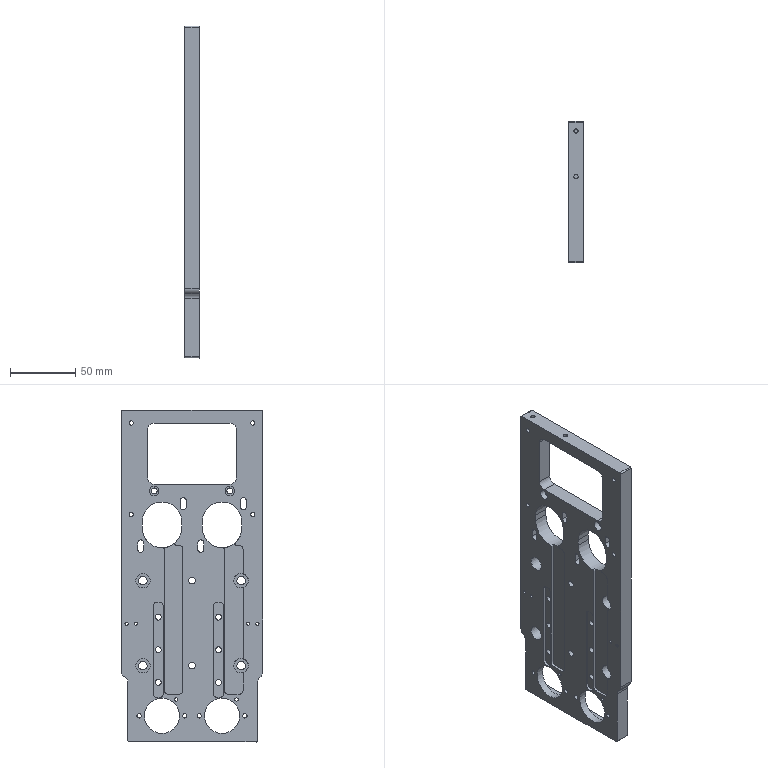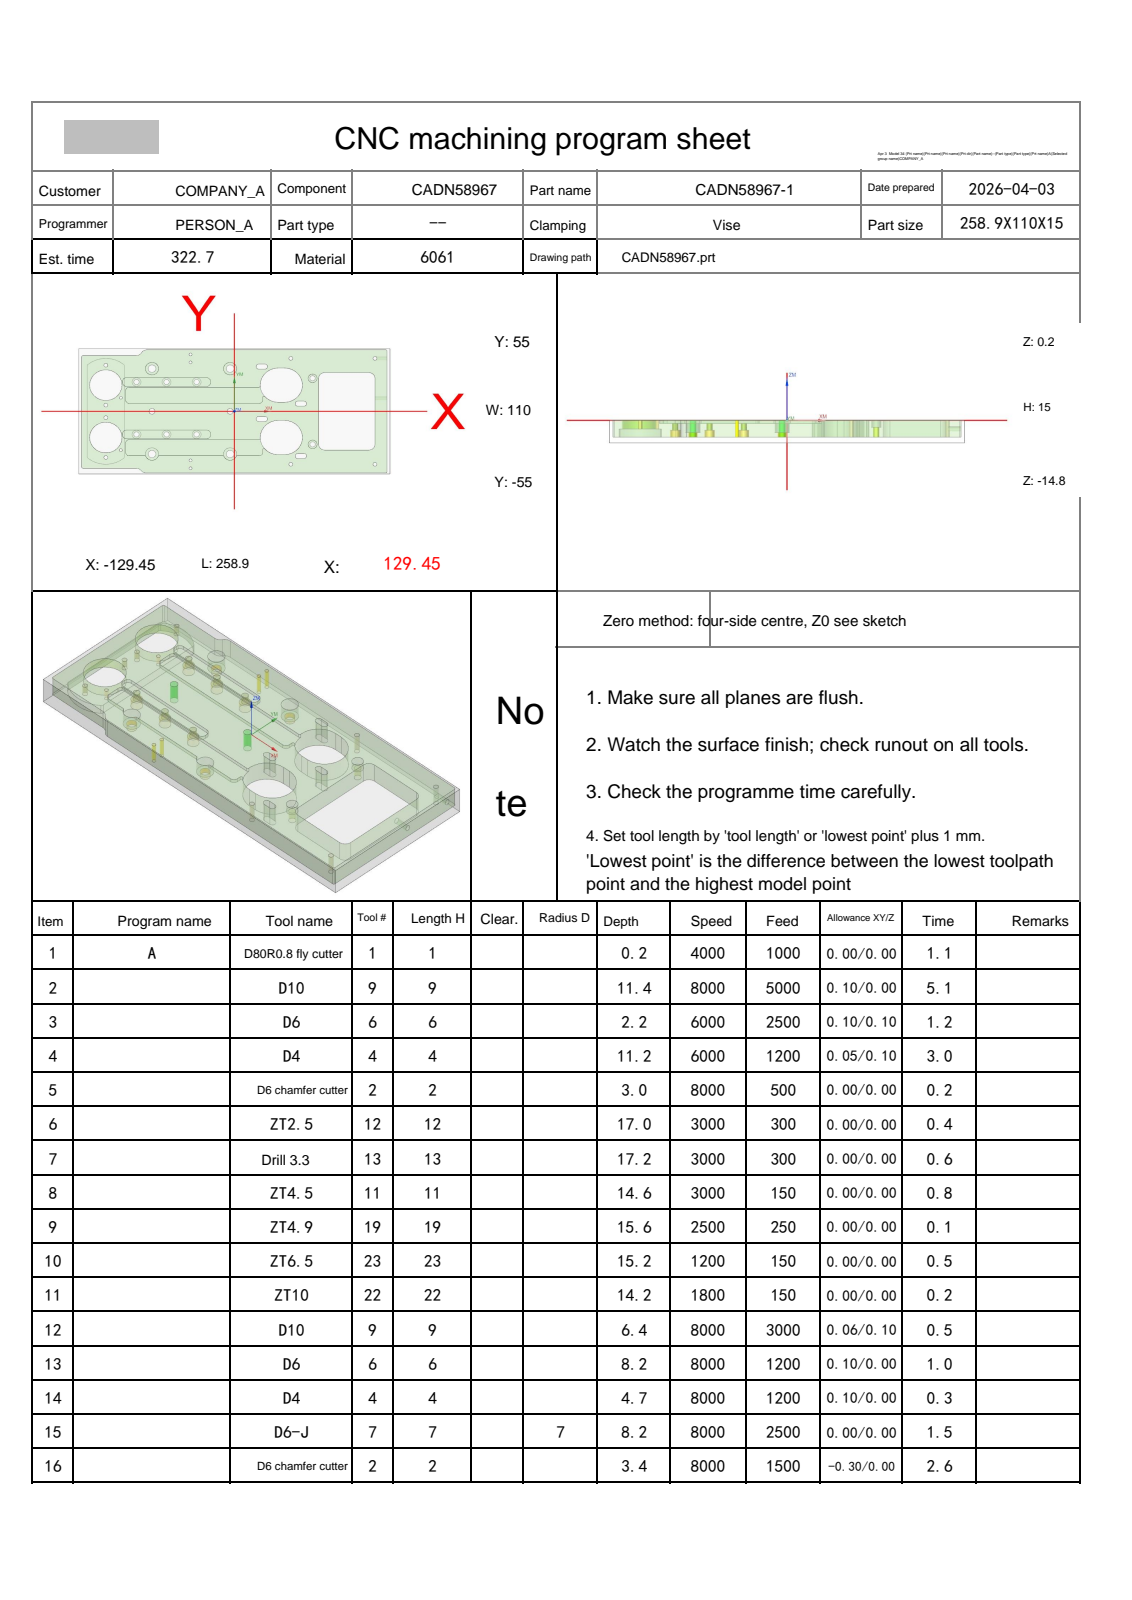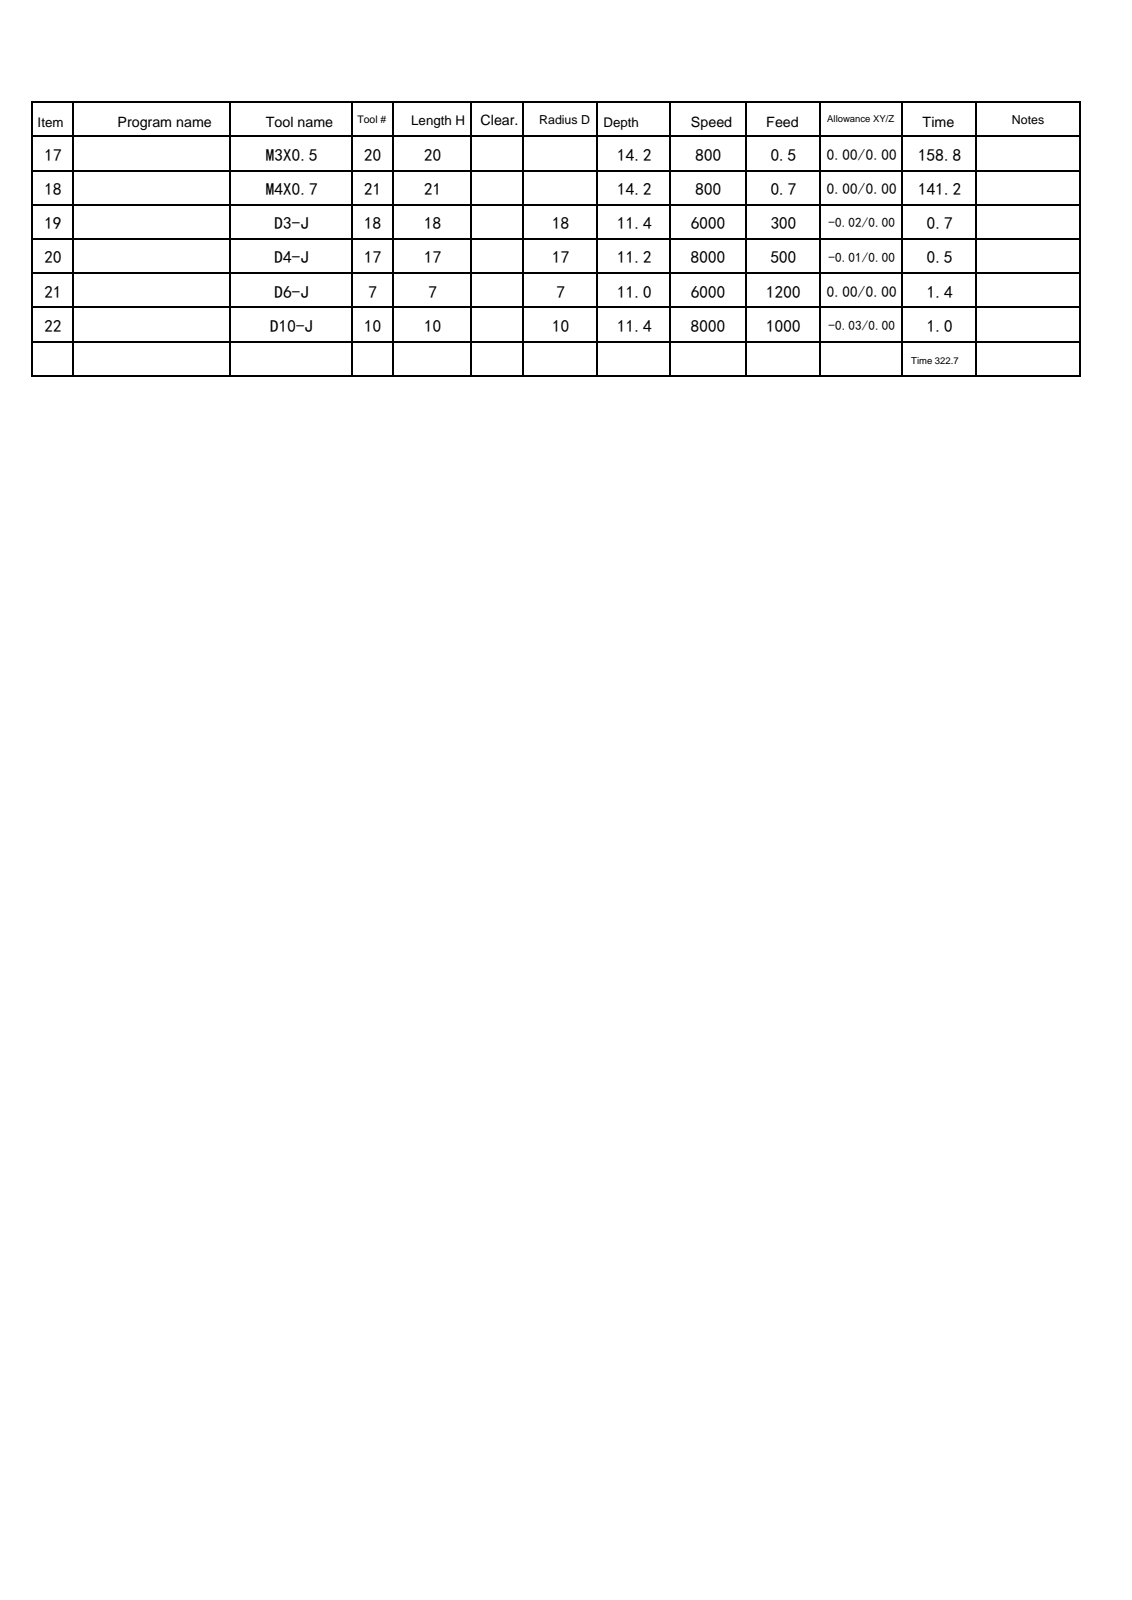NC program | NX | posted by the shop | part box 11 x 108 x 253.9 mm
Lines 1 to 910 of 8037:
%
O0001
(Machine time: 603.29 MIN)
(===Total Tool:17===)
(T1=D80R0.8 fly cutter D=80.  R=0.8  D-  H01 Z=0.    )
(T9=D10     D=10.  R=0.   D-  H09 Z=-11.2 )
(T6=D6      D=6.   R=0.   D-  H06 Z=-8.   )
(T4=D4      D=4.   R=0.   D-  H04 Z=-11.  )
(T2=D6 chamfer cutter   D=6.   R=0.   D-  H02 Z=-3.2  )
(T12=ZT2.5  D=2.5  DR_a=118 D-  H12 Z=-16.75)
(T13=drill 3.3  D=3.3  DR_a=118 D-  H13 Z=-17.  )
(T11=ZT4.5  D=4.5  DR_a=118 D-  H11 Z=-14.35)
(T19=ZT4.9  D=4.9  DR_a=120 D-  H19 Z=-15.41)
(T23=ZT6.5  D=6.5  DR_a=118 D-  H23 Z=-14.95)
(T22=ZT10   D=10.  DR_a=118 D-  H22 Z=-14.  )
(T7=D6-J    D=6.   R=0.   D7  H07 Z=-10.85)
(T20=M3X0.5 D=2.5  DR_a=180 D-  H20 Z=-14.  )
(T21=M4X0.7 D=3.3  DR_a=180 D-  H21 Z=-14.  )
(T18=D3-J   D=3.   R=0.   D18 H18 Z=-11.2 )
(T17=D4-J   D=4.   R=0.   D17 H17 Z=-11.  )
(T10=D10-J  D=10.  R=0.   D10 H10 Z=-11.2 )
G80 G90 G17 G49 G40
G91 G28 Z0
M01
N1 T01 M06
(D80R0.8 fly cutter  D=80. R=0.8 H=01 ce=0.00 di=0.00)
G00 G90 G54 X-171.95 Y47. M03 S4000
G43 H01 Z20.
M08
Z2.
G01 Z0.0 F1000.
X-166.95
X166.95
Y0.0
X-166.95
Y-47.
X166.95
X171.95
Z2.
G00 Z20.
G91 G28 Z0.0
M05
M09
G91 G28 Z0.0
M01
N2 T09 M06
(D10  D=10. R=0. H=09 ce=0.10 di=0.00)
G00 G90 G54 X26.2 Y-59.1 M03 S8000
G43 H09 Z20.
M08
Z.5
G01 X-73.55 Z.396 F5000.
G02 X-81.6 Y-55.1 Z.386 I0.0 J10.1
G01 X-125.95 Z.34
G02 X-132.05 Y-49. Z.33 I0.0 J6.1
G01 Y48. Z.229
G02 X-125.95 Y54.1 Z.219 I6.1 J0.0
G01 X-81.608 Z.173
G02 X-72.89 Y59.1 Z.162 I8.718 J-5.1
G01 X125.95 Z-.046
G02 X132.05 Y53. Z-.056 I0.0 J-6.1
G01 Y-53. Z-.166
G02 X125.95 Y-59.1 Z-.176 I-6.1 J0.0
G01 X-73.55 Z-.384
G02 X-81.6 Y-55.1 Z-.394 I0.0 J10.1
G01 X-125.95 Z-.44
G02 X-132.05 Y-49. Z-.45 I0.0 J6.1
G01 Y48. Z-.551
G02 X-125.95 Y54.1 Z-.561 I6.1 J0.0
G01 X-81.608 Z-.607
G02 X-72.89 Y59.1 Z-.618 I8.718 J-5.1
G01 X125.95 Z-.826
G02 X132.05 Y53. Z-.836 I0.0 J-6.1
G01 Y-53. Z-.946
G02 X125.95 Y-59.1 Z-.956 I-6.1 J0.0
G01 X-73.55 Z-1.164
G02 X-81.6 Y-55.1 Z-1.174 I0.0 J10.1
G01 X-125.95 Z-1.22
G02 X-132.05 Y-49. Z-1.23 I0.0 J6.1
G01 Y48. Z-1.331
G02 X-125.95 Y54.1 Z-1.341 I6.1 J0.0
G01 X-81.608 Z-1.387
G02 X-72.89 Y59.1 Z-1.398 I8.718 J-5.1
G01 X125.95 Z-1.606
G02 X132.05 Y53. Z-1.616 I0.0 J-6.1
G01 Y-53. Z-1.726
G02 X125.95 Y-59.1 Z-1.736 I-6.1 J0.0
G01 X-73.55 Z-1.944
G02 X-81.6 Y-55.1 Z-1.954 I0.0 J10.1
G01 X-125.95 Z-2.
G02 X-132.05 Y-49. Z-2.01 I0.0 J6.1
G01 Y48. Z-2.111
G02 X-125.95 Y54.1 Z-2.121 I6.1 J0.0
G01 X-81.608 Z-2.167
G02 X-72.89 Y59.1 Z-2.178 I8.718 J-5.1
G01 X125.95 Z-2.386
G02 X132.05 Y53. Z-2.396 I0.0 J-6.1
G01 Y-53. Z-2.506
G02 X125.95 Y-59.1 Z-2.516 I-6.1 J0.0
G01 X-73.55 Z-2.724
G02 X-81.6 Y-55.1 Z-2.734 I0.0 J10.1
G01 X-125.95 Z-2.78
G02 X-132.05 Y-49. Z-2.79 I0.0 J6.1
G01 Y48. Z-2.891
G02 X-125.95 Y54.1 Z-2.901 I6.1 J0.0
G01 X-81.608 Z-2.947
G02 X-72.89 Y59.1 Z-2.958 I8.718 J-5.1
G01 X125.95 Z-3.166
G02 X132.05 Y53. Z-3.176 I0.0 J-6.1
G01 Y-53. Z-3.286
G02 X125.95 Y-59.1 Z-3.296 I-6.1 J0.0
G01 X-73.55 Z-3.504
G02 X-81.6 Y-55.1 Z-3.514 I0.0 J10.1
G01 X-125.95 Z-3.56
G02 X-132.05 Y-49. Z-3.57 I0.0 J6.1
G01 Y48. Z-3.671
G02 X-125.95 Y54.1 Z-3.681 I6.1 J0.0
G01 X-81.608 Z-3.727
G02 X-72.89 Y59.1 Z-3.738 I8.718 J-5.1
G01 X125.95 Z-3.946
G02 X132.05 Y53. Z-3.956 I0.0 J-6.1
G01 Y-53. Z-4.066
G02 X125.95 Y-59.1 Z-4.076 I-6.1 J0.0
G01 X-73.55 Z-4.284
G02 X-81.6 Y-55.1 Z-4.294 I0.0 J10.1
G01 X-125.95 Z-4.34
G02 X-132.05 Y-49. Z-4.35 I0.0 J6.1
G01 Y48. Z-4.451
G02 X-125.95 Y54.1 Z-4.461 I6.1 J0.0
G01 X-81.608 Z-4.507
G02 X-72.89 Y59.1 Z-4.518 I8.718 J-5.1
G01 X125.95 Z-4.726
G02 X132.05 Y53. Z-4.736 I0.0 J-6.1
G01 Y-53. Z-4.846
G02 X125.95 Y-59.1 Z-4.856 I-6.1 J0.0
G01 X-73.55 Z-5.064
G02 X-81.6 Y-55.1 Z-5.074 I0.0 J10.1
G01 X-125.95 Z-5.12
G02 X-132.05 Y-49. Z-5.13 I0.0 J6.1
G01 Y48. Z-5.231
G02 X-125.95 Y54.1 Z-5.241 I6.1 J0.0
G01 X-81.608 Z-5.287
G02 X-72.89 Y59.1 Z-5.298 I8.718 J-5.1
G01 X125.95 Z-5.506
G02 X132.05 Y53. Z-5.516 I0.0 J-6.1
G01 Y-53. Z-5.626
G02 X125.95 Y-59.1 Z-5.636 I-6.1 J0.0
G01 X-73.55 Z-5.844
G02 X-81.6 Y-55.1 Z-5.854 I0.0 J10.1
G01 X-125.95 Z-5.9
G02 X-132.05 Y-49. Z-5.91 I0.0 J6.1
G01 Y48. Z-6.011
G02 X-125.95 Y54.1 Z-6.021 I6.1 J0.0
G01 X-81.608 Z-6.067
G02 X-72.89 Y59.1 Z-6.078 I8.718 J-5.1
G01 X125.95 Z-6.286
G02 X132.05 Y53. Z-6.296 I0.0 J-6.1
G01 Y-53. Z-6.406
G02 X125.95 Y-59.1 Z-6.416 I-6.1 J0.0
G01 X-73.55 Z-6.624
G02 X-81.6 Y-55.1 Z-6.634 I0.0 J10.1
G01 X-125.95 Z-6.68
G02 X-132.05 Y-49. Z-6.69 I0.0 J6.1
G01 Y48. Z-6.791
G02 X-125.95 Y54.1 Z-6.801 I6.1 J0.0
G01 X-81.608 Z-6.847
G02 X-72.89 Y59.1 Z-6.858 I8.718 J-5.1
G01 X125.95 Z-7.066
G02 X132.05 Y53. Z-7.076 I0.0 J-6.1
G01 Y-53. Z-7.186
G02 X125.95 Y-59.1 Z-7.196 I-6.1 J0.0
G01 X-73.55 Z-7.404
G02 X-81.6 Y-55.1 Z-7.414 I0.0 J10.1
G01 X-125.95 Z-7.46
G02 X-132.05 Y-49. Z-7.47 I0.0 J6.1
G01 Y48. Z-7.571
G02 X-125.95 Y54.1 Z-7.581 I6.1 J0.0
G01 X-81.608 Z-7.627
G02 X-72.89 Y59.1 Z-7.638 I8.718 J-5.1
G01 X125.95 Z-7.846
G02 X132.05 Y53. Z-7.856 I0.0 J-6.1
G01 Y-53. Z-7.966
G02 X125.95 Y-59.1 Z-7.976 I-6.1 J0.0
G01 X-73.55 Z-8.184
G02 X-81.6 Y-55.1 Z-8.194 I0.0 J10.1
G01 X-125.95 Z-8.24
G02 X-132.05 Y-49. Z-8.25 I0.0 J6.1
G01 Y48. Z-8.351
G02 X-125.95 Y54.1 Z-8.361 I6.1 J0.0
G01 X-81.608 Z-8.407
G02 X-72.89 Y59.1 Z-8.418 I8.718 J-5.1
G01 X125.95 Z-8.626
G02 X132.05 Y53. Z-8.636 I0.0 J-6.1
G01 Y-53. Z-8.746
G02 X125.95 Y-59.1 Z-8.756 I-6.1 J0.0
G01 X-73.55 Z-8.964
G02 X-81.6 Y-55.1 Z-8.974 I0.0 J10.1
G01 X-125.95 Z-9.02
G02 X-132.05 Y-49. Z-9.03 I0.0 J6.1
G01 Y48. Z-9.131
G02 X-125.95 Y54.1 Z-9.141 I6.1 J0.0
G01 X-81.608 Z-9.187
G02 X-72.89 Y59.1 Z-9.198 I8.718 J-5.1
G01 X125.95 Z-9.406
G02 X132.05 Y53. Z-9.416 I0.0 J-6.1
G01 Y-53. Z-9.526
G02 X125.95 Y-59.1 Z-9.536 I-6.1 J0.0
G01 X-73.55 Z-9.744
G02 X-81.6 Y-55.1 Z-9.754 I0.0 J10.1
G01 X-125.95 Z-9.8
G02 X-132.05 Y-49. Z-9.81 I0.0 J6.1
G01 Y48. Z-9.911
G02 X-125.95 Y54.1 Z-9.921 I6.1 J0.0
G01 X-81.608 Z-9.967
G02 X-72.89 Y59.1 Z-9.978 I8.718 J-5.1
G01 X125.95 Z-10.186
G02 X132.05 Y53. Z-10.196 I0.0 J-6.1
G01 Y-53. Z-10.306
G02 X125.95 Y-59.1 Z-10.316 I-6.1 J0.0
G01 X-73.55 Z-10.524
G02 X-81.6 Y-55.1 Z-10.534 I0.0 J10.1
G01 X-125.95 Z-10.58
G02 X-132.05 Y-49. Z-10.59 I0.0 J6.1
G01 Y48. Z-10.691
G02 X-125.95 Y54.1 Z-10.701 I6.1 J0.0
G01 X-81.608 Z-10.747
G02 X-72.89 Y59.1 Z-10.758 I8.718 J-5.1
G01 X125.95 Z-10.966
G02 X132.05 Y53. Z-10.976 I0.0 J-6.1
G01 Y-53. Z-11.086
G02 X125.95 Y-59.1 Z-11.096 I-6.1 J0.0
G01 X26.2 Z-11.2
X-73.55
G02 X-81.6 Y-55.1 I0.0 J10.1
G01 X-125.95
G02 X-132.05 Y-49. I0.0 J6.1
G01 Y48.
G02 X-125.95 Y54.1 I6.1 J0.0
G01 X-81.608
G02 X-72.89 Y59.1 I8.718 J-5.1
G01 X125.95
G02 X132.05 Y53. I0.0 J-6.1
G01 Y-53.
G02 X125.95 Y-59.1 I-6.1 J0.0
G01 X26.2
X25.7
Z-10.2
G00 Z20.
G00 G90 X4.46 Y-29.902 M03 S6000
Z20.
Z.5
G01 X-32.773 Z-.475 F3500.
X-85.35
Y-33.945
X-74.531
G02 X-68.918 Y-37.657 I0.0 J-6.1
G03 X-68.55 Y-37.9 I.368 J.157
X-68.182 Y-37.657 I0.0 J.4
G02 X-62.569 Y-33.945 I5.613 J-2.388
G01 X-9.531
G02 X-3.918 Y-37.657 I0.0 J-6.1
G03 X-3.55 Y-37.9 I.368 J.157
X-3.182 Y-37.657 I0.0 J.4
G02 X2.431 Y-33.945 I5.613 J-2.388
G01 X18.45
Y-33.734
G02 X19.803 Y-29.902 I6.1 J0.0
G01 X-32.773
X-33.273
Z.025
G00 Z.5
X4.46
Z.025
G01 X-32.773 Z-.95
X-85.35
Y-33.945
X-74.531
G02 X-68.918 Y-37.657 I0.0 J-6.1
G03 X-68.55 Y-37.9 I.368 J.157
X-68.182 Y-37.657 I0.0 J.4
G02 X-62.569 Y-33.945 I5.613 J-2.388
G01 X-9.531
G02 X-3.918 Y-37.657 I0.0 J-6.1
G03 X-3.55 Y-37.9 I.368 J.157
X-3.182 Y-37.657 I0.0 J.4
G02 X2.431 Y-33.945 I5.613 J-2.388
G01 X18.45
Y-33.734
G02 X19.803 Y-29.902 I6.1 J0.0
G01 X-32.773
X-33.273
Z-.45
G00 Z.025
X4.46
Z-.45
G01 X-32.773 Z-1.425
X-85.35
Y-33.945
X-74.531
G02 X-68.918 Y-37.657 I0.0 J-6.1
G03 X-68.55 Y-37.9 I.368 J.157
X-68.182 Y-37.657 I0.0 J.4
G02 X-62.569 Y-33.945 I5.613 J-2.388
G01 X-9.531
G02 X-3.918 Y-37.657 I0.0 J-6.1
G03 X-3.55 Y-37.9 I.368 J.157
X-3.182 Y-37.657 I0.0 J.4
G02 X2.431 Y-33.945 I5.613 J-2.388
G01 X18.45
Y-33.734
G02 X19.803 Y-29.902 I6.1 J0.0
G01 X-32.773
X-33.273
Z-.925
G00 Z-.45
X4.46
Z-.925
G01 X-32.773 Z-1.9
X-85.35
Y-33.945
X-74.531
G02 X-68.918 Y-37.657 I0.0 J-6.1
G03 X-68.55 Y-37.9 I.368 J.157
X-68.182 Y-37.657 I0.0 J.4
G02 X-62.569 Y-33.945 I5.613 J-2.388
G01 X-9.531
G02 X-3.918 Y-37.657 I0.0 J-6.1
G03 X-3.55 Y-37.9 I.368 J.157
X-3.182 Y-37.657 I0.0 J.4
G02 X2.431 Y-33.945 I5.613 J-2.388
G01 X18.45
Y-33.734
G02 X19.803 Y-29.902 I6.1 J0.0
G01 X-32.773
X-33.273
Z-1.4
G00 Z20.
G00 G90 X4.46 Y16.098 M03 S6000
Z20.
Z.5
G01 X-32.773 Z-.475 F3500.
X-85.35
Y12.055
X18.45
Y12.266
G02 X19.803 Y16.098 I6.1 J0.0
G01 X-32.773
X-33.273
Z.025
G00 Z.5
X4.46
Z.025
G01 X-32.773 Z-.95
X-85.35
Y12.055
X18.45
Y12.266
G02 X19.803 Y16.098 I6.1 J0.0
G01 X-32.773
X-33.273
Z-.45
G00 Z.025
X4.46
Z-.45
G01 X-32.773 Z-1.425
X-85.35
Y12.055
X18.45
Y12.266
G02 X19.803 Y16.098 I6.1 J0.0
G01 X-32.773
X-33.273
Z-.925
G00 Z-.45
X4.46
Z-.925
G01 X-32.773 Z-1.9
X-85.35
Y12.055
X18.45
Y12.266
G02 X19.803 Y16.098 I6.1 J0.0
G01 X-32.773
X-33.273
Z-1.4
G00 Z20.
G00 G90 X39.05 Y-33. M03 S6000
Z20.
Z.5
G01 X41.55 Z.483 F4000.
G03 X51.55 Y-23. Z.377 I0.0 J10.
X41.55 Y-13. Z.27 I-10. J0.0
G01 X36.55 Z.236
G03 X26.55 Y-23. Z.13 I0.0 J-10.
X36.55 Y-33. Z.023 I10. J0.0
G01 X41.55 Z-.01
G03 X51.55 Y-23. Z-.117 I0.0 J10.
X41.55 Y-13. Z-.223 I-10. J0.0
G01 X36.55 Z-.257
G03 X26.55 Y-23. Z-.364 I0.0 J-10.
X36.55 Y-33. Z-.47 I10. J0.0
G01 X41.55 Z-.504
G03 X51.55 Y-23. Z-.61 I0.0 J10.
X41.55 Y-13. Z-.717 I-10. J0.0
G01 X36.55 Z-.751
G03 X26.55 Y-23. Z-.857 I0.0 J-10.
X36.55 Y-33. Z-.963 I10. J0.0
G01 X41.55 Z-.997
G03 X51.55 Y-23. Z-1.104 I0.0 J10.
X41.55 Y-13. Z-1.21 I-10. J0.0
G01 X36.55 Z-1.244
G03 X26.55 Y-23. Z-1.351 I0.0 J-10.
X36.55 Y-33. Z-1.457 I10. J0.0
G01 X41.55 Z-1.491
G03 X51.55 Y-23. Z-1.597 I0.0 J10.
X41.55 Y-13. Z-1.704 I-10. J0.0
G01 X36.55 Z-1.738
G03 X26.55 Y-23. Z-1.844 I0.0 J-10.
X36.55 Y-33. Z-1.95 I10. J0.0
G01 X41.55 Z-1.984
G03 X51.55 Y-23. Z-2.091 I0.0 J10.
X41.55 Y-13. Z-2.197 I-10. J0.0
G01 X36.55 Z-2.231
G03 X26.55 Y-23. Z-2.338 I0.0 J-10.
X36.55 Y-33. Z-2.444 I10. J0.0
G01 X41.55 Z-2.478
G03 X51.55 Y-23. Z-2.584 I0.0 J10.
X41.55 Y-13. Z-2.691 I-10. J0.0
G01 X36.55 Z-2.725
G03 X26.55 Y-23. Z-2.831 I0.0 J-10.
X36.55 Y-33. Z-2.937 I10. J0.0
G01 X41.55 Z-2.971
G03 X51.55 Y-23. Z-3.078 I0.0 J10.
X41.55 Y-13. Z-3.184 I-10. J0.0
G01 X36.55 Z-3.218
G03 X26.55 Y-23. Z-3.324 I0.0 J-10.
X36.55 Y-33. Z-3.431 I10. J0.0
G01 X41.55 Z-3.465
G03 X51.55 Y-23. Z-3.571 I0.0 J10.
X41.55 Y-13. Z-3.678 I-10. J0.0
G01 X36.55 Z-3.712
G03 X26.55 Y-23. Z-3.818 I0.0 J-10.
X36.55 Y-33. Z-3.924 I10. J0.0
G01 X41.55 Z-3.958
G03 X51.55 Y-23. Z-4.065 I0.0 J10.
X41.55 Y-13. Z-4.171 I-10. J0.0
G01 X36.55 Z-4.205
G03 X26.55 Y-23. Z-4.311 I0.0 J-10.
X36.55 Y-33. Z-4.418 I10. J0.0
G01 X41.55 Z-4.452
G03 X51.55 Y-23. Z-4.558 I0.0 J10.
X41.55 Y-13. Z-4.665 I-10. J0.0
G01 X36.55 Z-4.698
G03 X26.55 Y-23. Z-4.805 I0.0 J-10.
X36.55 Y-33. Z-4.911 I10. J0.0
G01 X41.55 Z-4.945
G03 X51.55 Y-23. Z-5.052 I0.0 J10.
X41.55 Y-13. Z-5.158 I-10. J0.0
G01 X36.55 Z-5.192
G03 X26.55 Y-23. Z-5.298 I0.0 J-10.
X36.55 Y-33. Z-5.405 I10. J0.0
G01 X41.55 Z-5.439
G03 X51.55 Y-23. Z-5.545 I0.0 J10.
X41.55 Y-13. Z-5.652 I-10. J0.0
G01 X36.55 Z-5.685
G03 X26.55 Y-23. Z-5.792 I0.0 J-10.
X36.55 Y-33. Z-5.898 I10. J0.0
G01 X41.55 Z-5.932
G03 X51.55 Y-23. Z-6.039 I0.0 J10.
X41.55 Y-13. Z-6.145 I-10. J0.0
G01 X36.55 Z-6.179
G03 X26.55 Y-23. Z-6.285 I0.0 J-10.
X36.55 Y-33. Z-6.392 I10. J0.0
G01 X41.55 Z-6.426
G03 X51.55 Y-23. Z-6.532 I0.0 J10.
X41.55 Y-13. Z-6.638 I-10. J0.0
G01 X36.55 Z-6.672
G03 X26.55 Y-23. Z-6.779 I0.0 J-10.
X36.55 Y-33. Z-6.885 I10. J0.0
G01 X41.55 Z-6.919
G03 X51.55 Y-23. Z-7.026 I0.0 J10.
X41.55 Y-13. Z-7.132 I-10. J0.0
G01 X36.55 Z-7.166
G03 X26.55 Y-23. Z-7.272 I0.0 J-10.
X36.55 Y-33. Z-7.379 I10. J0.0
G01 X41.55 Z-7.413
G03 X51.55 Y-23. Z-7.519 I0.0 J10.
X41.55 Y-13. Z-7.625 I-10. J0.0
G01 X36.55 Z-7.659
G03 X26.55 Y-23. Z-7.766 I0.0 J-10.
X36.55 Y-33. Z-7.872 I10. J0.0
G01 X41.55 Z-7.906
G03 X51.55 Y-23. Z-8.013 I0.0 J10.
X41.55 Y-13. Z-8.119 I-10. J0.0
G01 X36.55 Z-8.153
G03 X26.55 Y-23. Z-8.259 I0.0 J-10.
X36.55 Y-33. Z-8.366 I10. J0.0
G01 X41.55 Z-8.4
G03 X51.55 Y-23. Z-8.506 I0.0 J10.
X41.55 Y-13. Z-8.612 I-10. J0.0
G01 X36.55 Z-8.646
G03 X26.55 Y-23. Z-8.753 I0.0 J-10.
X36.55 Y-33. Z-8.859 I10. J0.0
G01 X41.55 Z-8.893
G03 X51.55 Y-23. Z-8.999 I0.0 J10.
X41.55 Y-13. Z-9.106 I-10. J0.0
G01 X36.55 Z-9.14
G03 X26.55 Y-23. Z-9.246 I0.0 J-10.
X36.55 Y-33. Z-9.353 I10. J0.0
G01 X41.55 Z-9.387
G03 X51.55 Y-23. Z-9.493 I0.0 J10.
X41.55 Y-13. Z-9.599 I-10. J0.0
G01 X36.55 Z-9.633
G03 X26.55 Y-23. Z-9.74 I0.0 J-10.
X36.55 Y-33. Z-9.846 I10. J0.0
G01 X41.55 Z-9.88
G03 X51.55 Y-23. Z-9.986 I0.0 J10.
X41.55 Y-13. Z-10.093 I-10. J0.0
G01 X36.55 Z-10.127
G03 X26.55 Y-23. Z-10.233 I0.0 J-10.
X36.55 Y-33. Z-10.34 I10. J0.0
G01 X41.55 Z-10.373
G03 X51.55 Y-23. Z-10.48 I0.0 J10.
X41.55 Y-13. Z-10.586 I-10. J0.0
G01 X36.55 Z-10.62
G03 X26.55 Y-23. Z-10.727 I0.0 J-10.
X36.55 Y-33. Z-10.833 I10. J0.0
G01 X39.05 Z-10.85
X41.55
G03 X51.55 Y-23. I0.0 J10.
X41.55 Y-13. I-10. J0.0
G01 X36.55
G03 X26.55 Y-23. I0.0 J-10.
X36.55 Y-33. I10. J0.0
G01 X39.05
X39.55
Z-9.85
G00 Z20.
X39.05 Y33.
Z.5
G01 X36.55 Z.483
G03 X26.55 Y23. Z.377 I0.0 J-10.
X36.55 Y13. Z.27 I10. J0.0
G01 X41.55 Z.236
G03 X51.55 Y23. Z.13 I0.0 J10.
X41.55 Y33. Z.023 I-10. J0.0
G01 X36.55 Z-.01
G03 X26.55 Y23. Z-.117 I0.0 J-10.
X36.55 Y13. Z-.223 I10. J0.0
G01 X41.55 Z-.257
G03 X51.55 Y23. Z-.364 I0.0 J10.
X41.55 Y33. Z-.47 I-10. J0.0
G01 X36.55 Z-.504
G03 X26.55 Y23. Z-.61 I0.0 J-10.
X36.55 Y13. Z-.717 I10. J0.0
G01 X41.55 Z-.751
G03 X51.55 Y23. Z-.857 I0.0 J10.
X41.55 Y33. Z-.963 I-10. J0.0
G01 X36.55 Z-.997
G03 X26.55 Y23. Z-1.104 I0.0 J-10.
X36.55 Y13. Z-1.21 I10. J0.0
G01 X41.55 Z-1.244
G03 X51.55 Y23. Z-1.351 I0.0 J10.
X41.55 Y33. Z-1.457 I-10. J0.0
G01 X36.55 Z-1.491
G03 X26.55 Y23. Z-1.597 I0.0 J-10.
X36.55 Y13. Z-1.704 I10. J0.0
G01 X41.55 Z-1.738
G03 X51.55 Y23. Z-1.844 I0.0 J10.
X41.55 Y33. Z-1.95 I-10. J0.0
G01 X36.55 Z-1.984
G03 X26.55 Y23. Z-2.091 I0.0 J-10.
X36.55 Y13. Z-2.197 I10. J0.0
G01 X41.55 Z-2.231
G03 X51.55 Y23. Z-2.338 I0.0 J10.
X41.55 Y33. Z-2.444 I-10. J0.0
G01 X36.55 Z-2.478
G03 X26.55 Y23. Z-2.584 I0.0 J-10.
X36.55 Y13. Z-2.691 I10. J0.0
G01 X41.55 Z-2.725
G03 X51.55 Y23. Z-2.831 I0.0 J10.
X41.55 Y33. Z-2.937 I-10. J0.0
G01 X36.55 Z-2.971
G03 X26.55 Y23. Z-3.078 I0.0 J-10.
X36.55 Y13. Z-3.184 I10. J0.0
G01 X41.55 Z-3.218
G03 X51.55 Y23. Z-3.324 I0.0 J10.
X41.55 Y33. Z-3.431 I-10. J0.0
G01 X36.55 Z-3.465
G03 X26.55 Y23. Z-3.571 I0.0 J-10.
X36.55 Y13. Z-3.678 I10. J0.0
G01 X41.55 Z-3.712
G03 X51.55 Y23. Z-3.818 I0.0 J10.
X41.55 Y33. Z-3.924 I-10. J0.0
G01 X36.55 Z-3.958
G03 X26.55 Y23. Z-4.065 I0.0 J-10.
X36.55 Y13. Z-4.171 I10. J0.0
G01 X41.55 Z-4.205
G03 X51.55 Y23. Z-4.311 I0.0 J10.
X41.55 Y33. Z-4.418 I-10. J0.0
G01 X36.55 Z-4.452
G03 X26.55 Y23. Z-4.558 I0.0 J-10.
X36.55 Y13. Z-4.665 I10. J0.0
G01 X41.55 Z-4.698
G03 X51.55 Y23. Z-4.805 I0.0 J10.
X41.55 Y33. Z-4.911 I-10. J0.0
G01 X36.55 Z-4.945
G03 X26.55 Y23. Z-5.052 I0.0 J-10.
X36.55 Y13. Z-5.158 I10. J0.0
G01 X41.55 Z-5.192
G03 X51.55 Y23. Z-5.298 I0.0 J10.
X41.55 Y33. Z-5.405 I-10. J0.0
G01 X36.55 Z-5.439
G03 X26.55 Y23. Z-5.545 I0.0 J-10.
X36.55 Y13. Z-5.652 I10. J0.0
G01 X41.55 Z-5.685
G03 X51.55 Y23. Z-5.792 I0.0 J10.
X41.55 Y33. Z-5.898 I-10. J0.0
G01 X36.55 Z-5.932
G03 X26.55 Y23. Z-6.039 I0.0 J-10.
X36.55 Y13. Z-6.145 I10. J0.0
G01 X41.55 Z-6.179
G03 X51.55 Y23. Z-6.285 I0.0 J10.
X41.55 Y33. Z-6.392 I-10. J0.0
G01 X36.55 Z-6.426
G03 X26.55 Y23. Z-6.532 I0.0 J-10.
X36.55 Y13. Z-6.638 I10. J0.0
G01 X41.55 Z-6.672
G03 X51.55 Y23. Z-6.779 I0.0 J10.
X41.55 Y33. Z-6.885 I-10. J0.0
G01 X36.55 Z-6.919
G03 X26.55 Y23. Z-7.026 I0.0 J-10.
X36.55 Y13. Z-7.132 I10. J0.0
G01 X41.55 Z-7.166
G03 X51.55 Y23. Z-7.272 I0.0 J10.
X41.55 Y33. Z-7.379 I-10. J0.0
G01 X36.55 Z-7.413
G03 X26.55 Y23. Z-7.519 I0.0 J-10.
X36.55 Y13. Z-7.625 I10. J0.0
G01 X41.55 Z-7.659
G03 X51.55 Y23. Z-7.766 I0.0 J10.
X41.55 Y33. Z-7.872 I-10. J0.0
G01 X36.55 Z-7.906
G03 X26.55 Y23. Z-8.013 I0.0 J-10.
X36.55 Y13. Z-8.119 I10. J0.0
G01 X41.55 Z-8.153
G03 X51.55 Y23. Z-8.259 I0.0 J10.
X41.55 Y33. Z-8.366 I-10. J0.0
G01 X36.55 Z-8.4
G03 X26.55 Y23. Z-8.506 I0.0 J-10.
X36.55 Y13. Z-8.612 I10. J0.0
G01 X41.55 Z-8.646
G03 X51.55 Y23. Z-8.753 I0.0 J10.
X41.55 Y33. Z-8.859 I-10. J0.0
G01 X36.55 Z-8.893
G03 X26.55 Y23. Z-8.999 I0.0 J-10.
X36.55 Y13. Z-9.106 I10. J0.0
G01 X41.55 Z-9.14
G03 X51.55 Y23. Z-9.246 I0.0 J10.
X41.55 Y33. Z-9.353 I-10. J0.0
G01 X36.55 Z-9.387
G03 X26.55 Y23. Z-9.493 I0.0 J-10.
X36.55 Y13. Z-9.599 I10. J0.0
G01 X41.55 Z-9.633
G03 X51.55 Y23. Z-9.74 I0.0 J10.
X41.55 Y33. Z-9.846 I-10. J0.0
G01 X36.55 Z-9.88
G03 X26.55 Y23. Z-9.986 I0.0 J-10.
X36.55 Y13. Z-10.093 I10. J0.0
G01 X41.55 Z-10.127
G03 X51.55 Y23. Z-10.233 I0.0 J10.
X41.55 Y33. Z-10.34 I-10. J0.0
G01 X36.55 Z-10.373
G03 X26.55 Y23. Z-10.48 I0.0 J-10.
X36.55 Y13. Z-10.586 I10. J0.0
G01 X41.55 Z-10.62
G03 X51.55 Y23. Z-10.727 I0.0 J10.
X41.55 Y33. Z-10.833 I-10. J0.0
G01 X39.05 Z-10.85
X36.55
G03 X26.55 Y23. I0.0 J-10.
X36.55 Y13. I10. J0.0
G01 X41.55
G03 X51.55 Y23. I0.0 J10.
X41.55 Y33. I-10. J0.0
G01 X39.05
X38.55
Z-9.85
G00 Z20.
X111.85 Y0.0
Z.5
G01 Y28.9 Z.425
X75.15 Z.329
Y-28.9 Z.178
X111.85 Z.082
Y28.9 Z-.069
X75.15 Z-.165
Y-28.9 Z-.316
X111.85 Z-.411
Y28.9 Z-.562
X75.15 Z-.658
Y-28.9 Z-.809
X111.85 Z-.905
Y28.9 Z-1.056
X75.15 Z-1.152
Y-28.9 Z-1.303
X111.85 Z-1.398
Y28.9 Z-1.549
X75.15 Z-1.645
Y-28.9 Z-1.796
X111.85 Z-1.892
Y28.9 Z-2.043
X75.15 Z-2.139
Y-28.9 Z-2.29
X111.85 Z-2.385
Y28.9 Z-2.536
X75.15 Z-2.632
Y-28.9 Z-2.783
X111.85 Z-2.879
Y28.9 Z-3.03
X75.15 Z-3.126
Y-28.9 Z-3.277
X111.85 Z-3.372
Y28.9 Z-3.523
X75.15 Z-3.619
Y-28.9 Z-3.77
X111.85 Z-3.866
Y28.9 Z-4.017
X75.15 Z-4.113
Y-28.9 Z-4.264
X111.85 Z-4.359
Y28.9 Z-4.51
X75.15 Z-4.606
Y-28.9 Z-4.757
X111.85 Z-4.853
Y28.9 Z-5.004
X75.15 Z-5.1
Y-28.9 Z-5.25
X111.85 Z-5.346
Y28.9 Z-5.497
X75.15 Z-5.593
Y-28.9 Z-5.744
X111.85 Z-5.84
Y28.9 Z-5.991
X75.15 Z-6.086
Y-28.9 Z-6.237
X111.85 Z-6.333
Y28.9 Z-6.484
X75.15 Z-6.58
Y-28.9 Z-6.731
X111.85 Z-6.827
Y28.9 Z-6.978
X75.15 Z-7.073
Y-28.9 Z-7.224
X111.85 Z-7.32
Y28.9 Z-7.471
X75.15 Z-7.567
Y-28.9 Z-7.718
X111.85 Z-7.814
Y28.9 Z-7.965
X75.15 Z-8.06
Y-28.9 Z-8.211
X111.85 Z-8.307
Y28.9 Z-8.458
X75.15 Z-8.554
Y-28.9 Z-8.705
X111.85 Z-8.801
Y28.9 Z-8.952
X75.15 Z-9.047
Y-28.9 Z-9.198
X111.85 Z-9.294
Y28.9 Z-9.445
X75.15 Z-9.541
Y-28.9 Z-9.692
X111.85 Z-9.788
Y28.9 Z-9.939
X75.15 Z-10.034
Y-28.9 Z-10.185
X111.85 Z-10.281
Y28.9 Z-10.432
X75.15 Z-10.528
Y-28.9 Z-10.679
X111.85 Z-10.775
Y0.0 Z-10.85
Y28.9
X75.15
Y-28.9
X111.85
Y0.0
Y.5
Z-9.85
G00 Z20.
G91 G28 Z0.0
M05
M09
G91 G28 Z0.0
M01
N3 T06 M06
(D6  D=6. R=0. H=06 ce=0.10 di=0.10)
G00 G90 G54 X-56.45 Y-20.935 M03 S6000
G43 H06 Z20.
M08
Z.5
G01 X-23.015 Z.439 F2500.
Y-19.565 Z.436
X-89.885 Z.314
Y-20.935 Z.311
X-23.015 Z.189
Y-19.565 Z.186
X-89.885 Z.064
Y-20.935 Z.061
X-23.015 Z-.061
Y-19.565 Z-.064
X-89.885 Z-.186
Y-20.935 Z-.189
X-23.015 Z-.311
Y-19.565 Z-.314
X-89.885 Z-.436
Y-20.935 Z-.439
X-23.015 Z-.561
Y-19.565 Z-.564
X-89.885 Z-.686
Y-20.935 Z-.689
X-23.015 Z-.811
Y-19.565 Z-.814
X-89.885 Z-.936
Y-20.935 Z-.939
X-23.015 Z-1.061
Y-19.565 Z-1.064
X-89.885 Z-1.186
Y-20.935 Z-1.189
X-23.015 Z-1.311
Y-19.565 Z-1.314
X-89.885 Z-1.436
Y-20.935 Z-1.439
X-23.015 Z-1.561
Y-19.565 Z-1.564
X-89.885 Z-1.686
Y-20.935 Z-1.689
X-23.015 Z-1.811
Y-19.565 Z-1.814
X-89.885 Z-1.936
Y-20.935 Z-1.939
X-56.45 Z-2.
X-23.015
Y-19.565
X-89.885
Y-20.935
X-56.45
X-55.95
Z-1.
G00 Z20.
X-56.45 Y25.065
Z.5
G01 X-23.015 Z.439
Y26.435 Z.436
X-89.885 Z.314
Y25.065 Z.311
X-23.015 Z.189
Y26.435 Z.186
X-89.885 Z.064
Y25.065 Z.061
X-23.015 Z-.061
Y26.435 Z-.064
X-89.885 Z-.186
Y25.065 Z-.189
X-23.015 Z-.311
Y26.435 Z-.314
X-89.885 Z-.436
Y25.065 Z-.439
X-23.015 Z-.561
Y26.435 Z-.564
X-89.885 Z-.686
Y25.065 Z-.689
X-23.015 Z-.811
Y26.435 Z-.814
X-89.885 Z-.936
Y25.065 Z-.939
X-23.015 Z-1.061
Y26.435 Z-1.064
X-89.885 Z-1.186
Y25.065 Z-1.189
X-23.015 Z-1.311
Y26.435 Z-1.314
X-89.885 Z-1.436
Y25.065 Z-1.439
X-23.015 Z-1.561
Y26.435 Z-1.564
X-89.885 Z-1.686
Y25.065 Z-1.689
X-23.015 Z-1.811
Y26.435 Z-1.814
X-89.885 Z-1.936
Y25.065 Z-1.939
X-56.45 Z-2.
X-23.015
Y26.435
X-89.885
Y25.065
X-56.45
X-55.95
Z-1.
G00 Z20.
G91 G28 Z0.0
M05
M09
G91 G28 Z0.0
M01